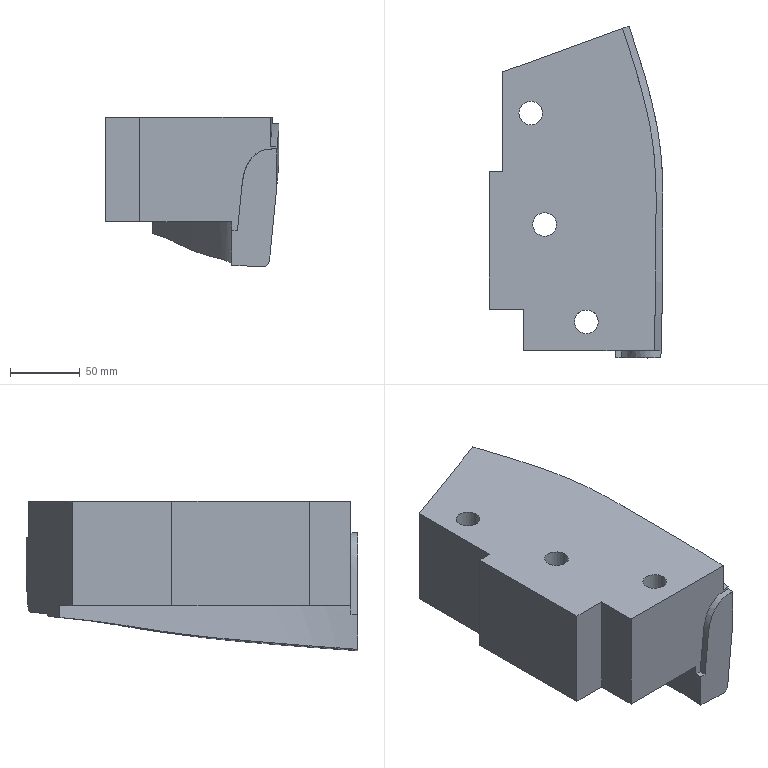Part | NX | features solid 2 | 1 solid | 116 faces | box 125.109 x 238.587 x 107.457 mm | volume 1908950 mm3 | spline 55 | cylinder 38 | plane 22 | cone 1 | commonest cylinder face diameters 6 x4 6.001 x3 16 x3 17 x3 25 x3 10.001 x2